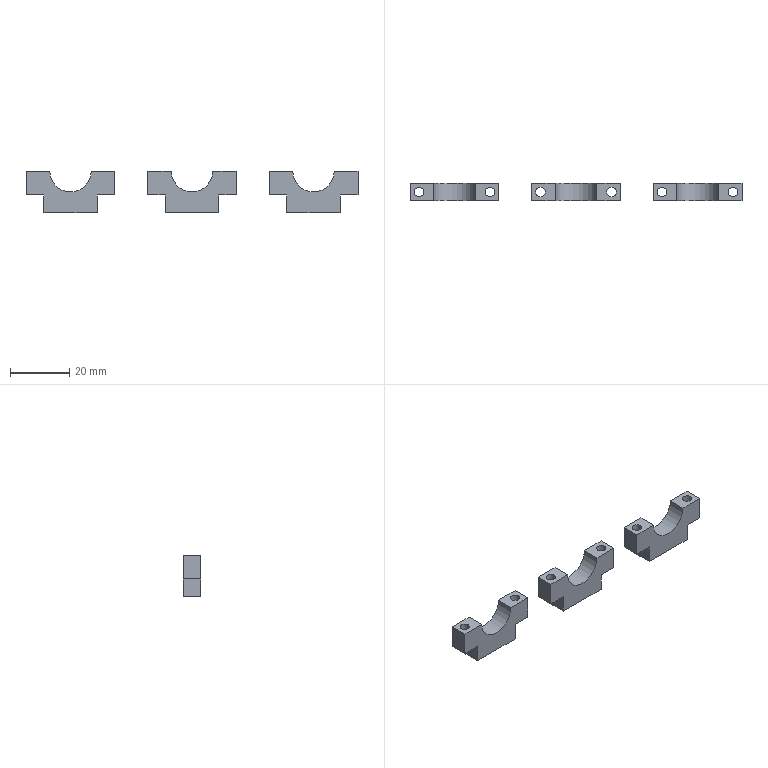Part | 3 solids | 42 faces | box 112 x 6 x 14 mm | volume 4493 mm3 | plane 33 | cylinder 9 | commonest cylinder face diameters 3.2 x6 14 x3
STEP:
#1=CARTESIAN_POINT('',(51.4,0.,-8.));
#2=VERTEX_POINT('',#1);
#3=CARTESIAN_POINT('',(53.,0.,-8.));
#4=DIRECTION('',(0.,0.,1.));
#5=DIRECTION('',(-1.,0.,0.));
#6=AXIS2_PLACEMENT_3D('',#3,#4,#5);
#7=CIRCLE('',#6,1.6);
#8=EDGE_CURVE('',#2,#2,#7,.T.);
#9=ORIENTED_EDGE('',*,*,#8,.F.);
#10=EDGE_LOOP('',(#9));
#11=FACE_BOUND('',#10,.T.);
#12=CARTESIAN_POINT('',(51.4,0.,0.));
#13=VERTEX_POINT('',#12);
#14=CARTESIAN_POINT('',(53.,0.,0.));
#15=DIRECTION('',(0.,0.,1.));
#16=DIRECTION('',(-1.,0.,0.));
#17=AXIS2_PLACEMENT_3D('',#14,#15,#16);
#18=CIRCLE('',#17,1.6);
#19=EDGE_CURVE('',#13,#13,#18,.T.);
#20=ORIENTED_EDGE('',*,*,#19,.T.);
#21=EDGE_LOOP('',(#20));
#22=FACE_BOUND('',#21,.T.);
#23=CARTESIAN_POINT('',(53.,0.,0.));
#24=DIRECTION('',(0.,0.,1.));
#25=DIRECTION('',(1.,0.,0.));
#26=AXIS2_PLACEMENT_3D('',#23,#24,#25);
#27=CYLINDRICAL_SURFACE('',#26,1.6);
#28=ADVANCED_FACE('',(#11,#22),#27,.F.);
#29=CARTESIAN_POINT('',(30.6,0.,-8.));
#30=VERTEX_POINT('',#29);
#31=CARTESIAN_POINT('',(29.,0.,-8.));
#32=DIRECTION('',(0.,0.,1.));
#33=DIRECTION('',(1.,0.,0.));
#34=AXIS2_PLACEMENT_3D('',#31,#32,#33);
#35=CIRCLE('',#34,1.6);
#36=EDGE_CURVE('',#30,#30,#35,.T.);
#37=ORIENTED_EDGE('',*,*,#36,.F.);
#38=EDGE_LOOP('',(#37));
#39=FACE_BOUND('',#38,.T.);
#40=CARTESIAN_POINT('',(30.6,0.,0.));
#41=VERTEX_POINT('',#40);
#42=CARTESIAN_POINT('',(29.,0.,0.));
#43=DIRECTION('',(0.,0.,1.));
#44=DIRECTION('',(1.,0.,0.));
#45=AXIS2_PLACEMENT_3D('',#42,#43,#44);
#46=CIRCLE('',#45,1.6);
#47=EDGE_CURVE('',#41,#41,#46,.T.);
#48=ORIENTED_EDGE('',*,*,#47,.T.);
#49=EDGE_LOOP('',(#48));
#50=FACE_BOUND('',#49,.T.);
#51=CARTESIAN_POINT('',(29.,0.,0.));
#52=DIRECTION('',(0.,0.,1.));
#53=DIRECTION('',(1.,0.,0.));
#54=AXIS2_PLACEMENT_3D('',#51,#52,#53);
#55=CYLINDRICAL_SURFACE('',#54,1.6);
#56=ADVANCED_FACE('',(#39,#50),#55,.F.);
#57=CARTESIAN_POINT('',(26.,3.,-8.));
#58=VERTEX_POINT('',#57);
#59=CARTESIAN_POINT('',(26.,3.,0.));
#60=VERTEX_POINT('',#59);
#61=CARTESIAN_POINT('',(26.,3.,-8.));
#62=DIRECTION('',(0.,0.,1.));
#63=VECTOR('',#62,1000.);
#64=LINE('',#61,#63);
#65=EDGE_CURVE('',#58,#60,#64,.T.);
#66=ORIENTED_EDGE('',*,*,#65,.T.);
#67=CARTESIAN_POINT('',(34.,3.,0.));
#68=VERTEX_POINT('',#67);
#69=CARTESIAN_POINT('',(41.,3.,0.));
#70=DIRECTION('',(1.,0.,0.));
#71=VECTOR('',#70,1000.);
#72=LINE('',#69,#71);
#73=EDGE_CURVE('',#60,#68,#72,.T.);
#74=ORIENTED_EDGE('',*,*,#73,.T.);
#75=CARTESIAN_POINT('',(48.,3.,0.));
#76=VERTEX_POINT('',#75);
#77=CARTESIAN_POINT('',(41.,3.,0.));
#78=DIRECTION('',(0.,-1.,0.));
#79=DIRECTION('',(-1.,0.,0.));
#80=AXIS2_PLACEMENT_3D('',#77,#78,#79);
#81=CIRCLE('',#80,7.);
#82=EDGE_CURVE('',#68,#76,#81,.T.);
#83=ORIENTED_EDGE('',*,*,#82,.T.);
#84=CARTESIAN_POINT('',(56.,3.,0.));
#85=VERTEX_POINT('',#84);
#86=CARTESIAN_POINT('',(48.,3.,0.));
#87=DIRECTION('',(1.,0.,0.));
#88=VECTOR('',#87,1000.);
#89=LINE('',#86,#88);
#90=EDGE_CURVE('',#76,#85,#89,.T.);
#91=ORIENTED_EDGE('',*,*,#90,.T.);
#92=CARTESIAN_POINT('',(56.,3.,-8.));
#93=VERTEX_POINT('',#92);
#94=CARTESIAN_POINT('',(56.,3.,0.));
#95=DIRECTION('',(0.,0.,-1.));
#96=VECTOR('',#95,1000.);
#97=LINE('',#94,#96);
#98=EDGE_CURVE('',#85,#93,#97,.T.);
#99=ORIENTED_EDGE('',*,*,#98,.T.);
#100=CARTESIAN_POINT('',(50.,3.,-8.));
#101=VERTEX_POINT('',#100);
#102=CARTESIAN_POINT('',(56.,3.,-8.));
#103=DIRECTION('',(-1.,0.,0.));
#104=VECTOR('',#103,1000.);
#105=LINE('',#102,#104);
#106=EDGE_CURVE('',#93,#101,#105,.T.);
#107=ORIENTED_EDGE('',*,*,#106,.T.);
#108=CARTESIAN_POINT('',(50.,3.,-14.));
#109=VERTEX_POINT('',#108);
#110=CARTESIAN_POINT('',(50.,3.,-14.));
#111=DIRECTION('',(0.,0.,1.));
#112=VECTOR('',#111,1000.);
#113=LINE('',#110,#112);
#114=EDGE_CURVE('',#109,#101,#113,.T.);
#115=ORIENTED_EDGE('',*,*,#114,.F.);
#116=CARTESIAN_POINT('',(32.,3.,-14.));
#117=VERTEX_POINT('',#116);
#118=CARTESIAN_POINT('',(50.,3.,-14.));
#119=DIRECTION('',(-1.,0.,0.));
#120=VECTOR('',#119,1000.);
#121=LINE('',#118,#120);
#122=EDGE_CURVE('',#109,#117,#121,.T.);
#123=ORIENTED_EDGE('',*,*,#122,.T.);
#124=CARTESIAN_POINT('',(32.,3.,-8.));
#125=VERTEX_POINT('',#124);
#126=CARTESIAN_POINT('',(32.,3.,-8.));
#127=DIRECTION('',(0.,0.,-1.));
#128=VECTOR('',#127,1000.);
#129=LINE('',#126,#128);
#130=EDGE_CURVE('',#125,#117,#129,.T.);
#131=ORIENTED_EDGE('',*,*,#130,.F.);
#132=CARTESIAN_POINT('',(50.,3.,-8.));
#133=DIRECTION('',(1.,0.,0.));
#134=VECTOR('',#133,1000.);
#135=LINE('',#132,#134);
#136=EDGE_CURVE('',#58,#125,#135,.T.);
#137=ORIENTED_EDGE('',*,*,#136,.F.);
#138=EDGE_LOOP('',(#66,#74,#83,#91,#99,#107,#115,#123,#131,#137));
#139=FACE_BOUND('',#138,.T.);
#140=CARTESIAN_POINT('',(41.,3.,0.));
#141=DIRECTION('',(0.,1.,0.));
#142=DIRECTION('',(1.,0.,0.));
#143=AXIS2_PLACEMENT_3D('',#140,#141,#142);
#144=PLANE('',#143);
#145=ADVANCED_FACE('',(#139),#144,.T.);
#146=CARTESIAN_POINT('',(26.,-3.,-8.));
#147=VERTEX_POINT('',#146);
#148=CARTESIAN_POINT('',(26.,-3.,0.));
#149=VERTEX_POINT('',#148);
#150=CARTESIAN_POINT('',(26.,-3.,-8.));
#151=DIRECTION('',(0.,0.,1.));
#152=VECTOR('',#151,1000.);
#153=LINE('',#150,#152);
#154=EDGE_CURVE('',#147,#149,#153,.T.);
#155=ORIENTED_EDGE('',*,*,#154,.T.);
#156=CARTESIAN_POINT('',(26.,-3.,0.));
#157=DIRECTION('',(0.,1.,0.));
#158=VECTOR('',#157,1000.);
#159=LINE('',#156,#158);
#160=EDGE_CURVE('',#149,#60,#159,.T.);
#161=ORIENTED_EDGE('',*,*,#160,.T.);
#162=ORIENTED_EDGE('',*,*,#65,.F.);
#163=CARTESIAN_POINT('',(26.,3.,-8.));
#164=DIRECTION('',(0.,1.,0.));
#165=VECTOR('',#164,1000.);
#166=LINE('',#163,#165);
#167=EDGE_CURVE('',#147,#58,#166,.T.);
#168=ORIENTED_EDGE('',*,*,#167,.F.);
#169=EDGE_LOOP('',(#155,#161,#162,#168));
#170=FACE_BOUND('',#169,.T.);
#171=CARTESIAN_POINT('',(26.,-3.,-14.));
#172=DIRECTION('',(-1.,0.,0.));
#173=DIRECTION('',(0.,0.,1.));
#174=AXIS2_PLACEMENT_3D('',#171,#172,#173);
#175=PLANE('',#174);
#176=ADVANCED_FACE('',(#170),#175,.T.);
#177=ORIENTED_EDGE('',*,*,#47,.F.);
#178=EDGE_LOOP('',(#177));
#179=FACE_BOUND('',#178,.T.);
#180=CARTESIAN_POINT('',(34.,-3.,0.));
#181=VERTEX_POINT('',#180);
#182=CARTESIAN_POINT('',(34.,-3.,0.));
#183=DIRECTION('',(0.,1.,0.));
#184=VECTOR('',#183,1000.);
#185=LINE('',#182,#184);
#186=EDGE_CURVE('',#181,#68,#185,.T.);
#187=ORIENTED_EDGE('',*,*,#186,.T.);
#188=ORIENTED_EDGE('',*,*,#73,.F.);
#189=ORIENTED_EDGE('',*,*,#160,.F.);
#190=CARTESIAN_POINT('',(48.,-3.,0.));
#191=DIRECTION('',(1.,0.,0.));
#192=VECTOR('',#191,1000.);
#193=LINE('',#190,#192);
#194=EDGE_CURVE('',#149,#181,#193,.T.);
#195=ORIENTED_EDGE('',*,*,#194,.T.);
#196=EDGE_LOOP('',(#187,#188,#189,#195));
#197=FACE_BOUND('',#196,.T.);
#198=CARTESIAN_POINT('',(48.,-3.,0.));
#199=DIRECTION('',(0.,0.,1.));
#200=DIRECTION('',(1.,0.,0.));
#201=AXIS2_PLACEMENT_3D('',#198,#199,#200);
#202=PLANE('',#201);
#203=ADVANCED_FACE('',(#179,#197),#202,.T.);
#204=CARTESIAN_POINT('',(48.,-3.,0.));
#205=VERTEX_POINT('',#204);
#206=CARTESIAN_POINT('',(48.,-3.,0.));
#207=DIRECTION('',(0.,1.,0.));
#208=VECTOR('',#207,1000.);
#209=LINE('',#206,#208);
#210=EDGE_CURVE('',#205,#76,#209,.T.);
#211=ORIENTED_EDGE('',*,*,#210,.T.);
#212=ORIENTED_EDGE('',*,*,#82,.F.);
#213=ORIENTED_EDGE('',*,*,#186,.F.);
#214=CARTESIAN_POINT('',(41.,-3.,0.));
#215=DIRECTION('',(0.,-1.,0.));
#216=DIRECTION('',(-1.,0.,0.));
#217=AXIS2_PLACEMENT_3D('',#214,#215,#216);
#218=CIRCLE('',#217,7.);
#219=EDGE_CURVE('',#181,#205,#218,.T.);
#220=ORIENTED_EDGE('',*,*,#219,.T.);
#221=EDGE_LOOP('',(#211,#212,#213,#220));
#222=FACE_BOUND('',#221,.T.);
#223=CARTESIAN_POINT('',(41.,-3.,0.));
#224=DIRECTION('',(0.,1.,0.));
#225=DIRECTION('',(1.,0.,0.));
#226=AXIS2_PLACEMENT_3D('',#223,#224,#225);
#227=CYLINDRICAL_SURFACE('',#226,7.);
#228=ADVANCED_FACE('',(#222),#227,.F.);
#229=ORIENTED_EDGE('',*,*,#19,.F.);
#230=EDGE_LOOP('',(#229));
#231=FACE_BOUND('',#230,.T.);
#232=CARTESIAN_POINT('',(56.,-3.,0.));
#233=VERTEX_POINT('',#232);
#234=CARTESIAN_POINT('',(56.,-3.,0.));
#235=DIRECTION('',(0.,1.,0.));
#236=VECTOR('',#235,1000.);
#237=LINE('',#234,#236);
#238=EDGE_CURVE('',#233,#85,#237,.T.);
#239=ORIENTED_EDGE('',*,*,#238,.T.);
#240=ORIENTED_EDGE('',*,*,#90,.F.);
#241=ORIENTED_EDGE('',*,*,#210,.F.);
#242=CARTESIAN_POINT('',(48.,-3.,0.));
#243=DIRECTION('',(1.,0.,0.));
#244=VECTOR('',#243,1000.);
#245=LINE('',#242,#244);
#246=EDGE_CURVE('',#205,#233,#245,.T.);
#247=ORIENTED_EDGE('',*,*,#246,.T.);
#248=EDGE_LOOP('',(#239,#240,#241,#247));
#249=FACE_BOUND('',#248,.T.);
#250=CARTESIAN_POINT('',(48.,-3.,0.));
#251=DIRECTION('',(0.,0.,1.));
#252=DIRECTION('',(1.,0.,0.));
#253=AXIS2_PLACEMENT_3D('',#250,#251,#252);
#254=PLANE('',#253);
#255=ADVANCED_FACE('',(#231,#249),#254,.T.);
#256=ORIENTED_EDGE('',*,*,#98,.F.);
#257=ORIENTED_EDGE('',*,*,#238,.F.);
#258=CARTESIAN_POINT('',(56.,-3.,-8.));
#259=VERTEX_POINT('',#258);
#260=CARTESIAN_POINT('',(56.,-3.,0.));
#261=DIRECTION('',(0.,0.,-1.));
#262=VECTOR('',#261,1000.);
#263=LINE('',#260,#262);
#264=EDGE_CURVE('',#233,#259,#263,.T.);
#265=ORIENTED_EDGE('',*,*,#264,.T.);
#266=CARTESIAN_POINT('',(56.,-3.,-8.));
#267=DIRECTION('',(0.,1.,0.));
#268=VECTOR('',#267,1000.);
#269=LINE('',#266,#268);
#270=EDGE_CURVE('',#259,#93,#269,.T.);
#271=ORIENTED_EDGE('',*,*,#270,.T.);
#272=EDGE_LOOP('',(#256,#257,#265,#271));
#273=FACE_BOUND('',#272,.T.);
#274=CARTESIAN_POINT('',(56.,-3.,0.));
#275=DIRECTION('',(1.,0.,0.));
#276=DIRECTION('',(0.,0.,-1.));
#277=AXIS2_PLACEMENT_3D('',#274,#275,#276);
#278=PLANE('',#277);
#279=ADVANCED_FACE('',(#273),#278,.T.);
#280=ORIENTED_EDGE('',*,*,#8,.T.);
#281=EDGE_LOOP('',(#280));
#282=FACE_BOUND('',#281,.T.);
#283=CARTESIAN_POINT('',(50.,-3.,-8.));
#284=VERTEX_POINT('',#283);
#285=CARTESIAN_POINT('',(50.,3.,-8.));
#286=DIRECTION('',(0.,-1.,0.));
#287=VECTOR('',#286,1000.);
#288=LINE('',#285,#287);
#289=EDGE_CURVE('',#101,#284,#288,.T.);
#290=ORIENTED_EDGE('',*,*,#289,.F.);
#291=ORIENTED_EDGE('',*,*,#106,.F.);
#292=ORIENTED_EDGE('',*,*,#270,.F.);
#293=CARTESIAN_POINT('',(56.,-3.,-8.));
#294=DIRECTION('',(-1.,0.,0.));
#295=VECTOR('',#294,1000.);
#296=LINE('',#293,#295);
#297=EDGE_CURVE('',#259,#284,#296,.T.);
#298=ORIENTED_EDGE('',*,*,#297,.T.);
#299=EDGE_LOOP('',(#290,#291,#292,#298));
#300=FACE_BOUND('',#299,.T.);
#301=CARTESIAN_POINT('',(50.,3.,-8.));
#302=DIRECTION('',(0.,0.,1.));
#303=DIRECTION('',(1.,0.,0.));
#304=AXIS2_PLACEMENT_3D('',#301,#302,#303);
#305=PLANE('',#304);
#306=ADVANCED_FACE('',(#282,#300),#305,.F.);
#307=CARTESIAN_POINT('',(50.,-3.,-14.));
#308=VERTEX_POINT('',#307);
#309=CARTESIAN_POINT('',(50.,-3.,-14.));
#310=DIRECTION('',(0.,1.,0.));
#311=VECTOR('',#310,1000.);
#312=LINE('',#309,#311);
#313=EDGE_CURVE('',#308,#109,#312,.T.);
#314=ORIENTED_EDGE('',*,*,#313,.T.);
#315=ORIENTED_EDGE('',*,*,#114,.T.);
#316=ORIENTED_EDGE('',*,*,#289,.T.);
#317=CARTESIAN_POINT('',(50.,-3.,-14.));
#318=DIRECTION('',(0.,0.,1.));
#319=VECTOR('',#318,1000.);
#320=LINE('',#317,#319);
#321=EDGE_CURVE('',#308,#284,#320,.T.);
#322=ORIENTED_EDGE('',*,*,#321,.F.);
#323=EDGE_LOOP('',(#314,#315,#316,#322));
#324=FACE_BOUND('',#323,.T.);
#325=CARTESIAN_POINT('',(50.,3.,-14.));
#326=DIRECTION('',(-1.,0.,0.));
#327=DIRECTION('',(0.,0.,1.));
#328=AXIS2_PLACEMENT_3D('',#325,#326,#327);
#329=PLANE('',#328);
#330=ADVANCED_FACE('',(#324),#329,.F.);
#331=ORIENTED_EDGE('',*,*,#122,.F.);
#332=ORIENTED_EDGE('',*,*,#313,.F.);
#333=CARTESIAN_POINT('',(32.,-3.,-14.));
#334=VERTEX_POINT('',#333);
#335=CARTESIAN_POINT('',(50.,-3.,-14.));
#336=DIRECTION('',(-1.,0.,0.));
#337=VECTOR('',#336,1000.);
#338=LINE('',#335,#337);
#339=EDGE_CURVE('',#308,#334,#338,.T.);
#340=ORIENTED_EDGE('',*,*,#339,.T.);
#341=CARTESIAN_POINT('',(32.,-3.,-14.));
#342=DIRECTION('',(0.,1.,0.));
#343=VECTOR('',#342,1000.);
#344=LINE('',#341,#343);
#345=EDGE_CURVE('',#334,#117,#344,.T.);
#346=ORIENTED_EDGE('',*,*,#345,.T.);
#347=EDGE_LOOP('',(#331,#332,#340,#346));
#348=FACE_BOUND('',#347,.T.);
#349=CARTESIAN_POINT('',(56.,-3.,-14.));
#350=DIRECTION('',(0.,0.,-1.));
#351=DIRECTION('',(-1.,0.,0.));
#352=AXIS2_PLACEMENT_3D('',#349,#350,#351);
#353=PLANE('',#352);
#354=ADVANCED_FACE('',(#348),#353,.T.);
#355=CARTESIAN_POINT('',(32.,-3.,-8.));
#356=VERTEX_POINT('',#355);
#357=CARTESIAN_POINT('',(32.,3.,-8.));
#358=DIRECTION('',(0.,-1.,0.));
#359=VECTOR('',#358,1000.);
#360=LINE('',#357,#359);
#361=EDGE_CURVE('',#125,#356,#360,.T.);
#362=ORIENTED_EDGE('',*,*,#361,.F.);
#363=ORIENTED_EDGE('',*,*,#130,.T.);
#364=ORIENTED_EDGE('',*,*,#345,.F.);
#365=CARTESIAN_POINT('',(32.,-3.,-8.));
#366=DIRECTION('',(0.,0.,-1.));
#367=VECTOR('',#366,1000.);
#368=LINE('',#365,#367);
#369=EDGE_CURVE('',#356,#334,#368,.T.);
#370=ORIENTED_EDGE('',*,*,#369,.F.);
#371=EDGE_LOOP('',(#362,#363,#364,#370));
#372=FACE_BOUND('',#371,.T.);
#373=CARTESIAN_POINT('',(32.,3.,-8.));
#374=DIRECTION('',(1.,0.,0.));
#375=DIRECTION('',(0.,0.,-1.));
#376=AXIS2_PLACEMENT_3D('',#373,#374,#375);
#377=PLANE('',#376);
#378=ADVANCED_FACE('',(#372),#377,.F.);
#379=ORIENTED_EDGE('',*,*,#36,.T.);
#380=EDGE_LOOP('',(#379));
#381=FACE_BOUND('',#380,.T.);
#382=ORIENTED_EDGE('',*,*,#167,.T.);
#383=ORIENTED_EDGE('',*,*,#136,.T.);
#384=ORIENTED_EDGE('',*,*,#361,.T.);
#385=CARTESIAN_POINT('',(41.,-3.,-8.));
#386=DIRECTION('',(1.,0.,0.));
#387=VECTOR('',#386,1000.);
#388=LINE('',#385,#387);
#389=EDGE_CURVE('',#147,#356,#388,.T.);
#390=ORIENTED_EDGE('',*,*,#389,.F.);
#391=EDGE_LOOP('',(#382,#383,#384,#390));
#392=FACE_BOUND('',#391,.T.);
#393=CARTESIAN_POINT('',(50.,3.,-8.));
#394=DIRECTION('',(0.,0.,1.));
#395=DIRECTION('',(1.,0.,0.));
#396=AXIS2_PLACEMENT_3D('',#393,#394,#395);
#397=PLANE('',#396);
#398=ADVANCED_FACE('',(#381,#392),#397,.F.);
#399=ORIENTED_EDGE('',*,*,#369,.T.);
#400=ORIENTED_EDGE('',*,*,#339,.F.);
#401=ORIENTED_EDGE('',*,*,#321,.T.);
#402=ORIENTED_EDGE('',*,*,#297,.F.);
#403=ORIENTED_EDGE('',*,*,#264,.F.);
#404=ORIENTED_EDGE('',*,*,#246,.F.);
#405=ORIENTED_EDGE('',*,*,#219,.F.);
#406=ORIENTED_EDGE('',*,*,#194,.F.);
#407=ORIENTED_EDGE('',*,*,#154,.F.);
#408=ORIENTED_EDGE('',*,*,#389,.T.);
#409=EDGE_LOOP('',(#399,#400,#401,#402,#403,#404,#405,#406,#407,#408));
#410=FACE_BOUND('',#409,.T.);
#411=CARTESIAN_POINT('',(41.,-3.,0.));
#412=DIRECTION('',(0.,1.,0.));
#413=DIRECTION('',(1.,0.,0.));
#414=AXIS2_PLACEMENT_3D('',#411,#412,#413);
#415=PLANE('',#414);
#416=ADVANCED_FACE('',(#410),#415,.F.);
#417=CLOSED_SHELL('',(#28,#56,#145,#176,#203,#228,#255,#279,#306,#330,#354,#378,#398,#416));
#418=MANIFOLD_SOLID_BREP('',#417);
#419=CARTESIAN_POINT('',(10.4,0.,-8.));
#420=VERTEX_POINT('',#419);
#421=CARTESIAN_POINT('',(12.,0.,-8.));
#422=DIRECTION('',(0.,0.,1.));
#423=DIRECTION('',(-1.,0.,0.));
#424=AXIS2_PLACEMENT_3D('',#421,#422,#423);
#425=CIRCLE('',#424,1.6);
#426=EDGE_CURVE('',#420,#420,#425,.T.);
#427=ORIENTED_EDGE('',*,*,#426,.F.);
#428=EDGE_LOOP('',(#427));
#429=FACE_BOUND('',#428,.T.);
#430=CARTESIAN_POINT('',(10.4,0.,0.));
#431=VERTEX_POINT('',#430);
#432=CARTESIAN_POINT('',(12.,0.,0.));
#433=DIRECTION('',(0.,0.,1.));
#434=DIRECTION('',(-1.,0.,0.));
#435=AXIS2_PLACEMENT_3D('',#432,#433,#434);
#436=CIRCLE('',#435,1.6);
#437=EDGE_CURVE('',#431,#431,#436,.T.);
#438=ORIENTED_EDGE('',*,*,#437,.T.);
#439=EDGE_LOOP('',(#438));
#440=FACE_BOUND('',#439,.T.);
#441=CARTESIAN_POINT('',(12.,0.,0.));
#442=DIRECTION('',(0.,0.,1.));
#443=DIRECTION('',(1.,0.,0.));
#444=AXIS2_PLACEMENT_3D('',#441,#442,#443);
#445=CYLINDRICAL_SURFACE('',#444,1.6);
#446=ADVANCED_FACE('',(#429,#440),#445,.F.);
#447=CARTESIAN_POINT('',(-10.4,0.,-8.));
#448=VERTEX_POINT('',#447);
#449=CARTESIAN_POINT('',(-12.,0.,-8.));
#450=DIRECTION('',(0.,0.,1.));
#451=DIRECTION('',(1.,0.,0.));
#452=AXIS2_PLACEMENT_3D('',#449,#450,#451);
#453=CIRCLE('',#452,1.6);
#454=EDGE_CURVE('',#448,#448,#453,.T.);
#455=ORIENTED_EDGE('',*,*,#454,.F.);
#456=EDGE_LOOP('',(#455));
#457=FACE_BOUND('',#456,.T.);
#458=CARTESIAN_POINT('',(-10.4,0.,0.));
#459=VERTEX_POINT('',#458);
#460=CARTESIAN_POINT('',(-12.,0.,0.));
#461=DIRECTION('',(0.,0.,1.));
#462=DIRECTION('',(1.,0.,0.));
#463=AXIS2_PLACEMENT_3D('',#460,#461,#462);
#464=CIRCLE('',#463,1.6);
#465=EDGE_CURVE('',#459,#459,#464,.T.);
#466=ORIENTED_EDGE('',*,*,#465,.T.);
#467=EDGE_LOOP('',(#466));
#468=FACE_BOUND('',#467,.T.);
#469=CARTESIAN_POINT('',(-12.,0.,0.));
#470=DIRECTION('',(0.,0.,1.));
#471=DIRECTION('',(1.,0.,0.));
#472=AXIS2_PLACEMENT_3D('',#469,#470,#471);
#473=CYLINDRICAL_SURFACE('',#472,1.6);
#474=ADVANCED_FACE('',(#457,#468),#473,.F.);
#475=CARTESIAN_POINT('',(-15.,3.,-8.));
#476=VERTEX_POINT('',#475);
#477=CARTESIAN_POINT('',(-15.,3.,0.));
#478=VERTEX_POINT('',#477);
#479=CARTESIAN_POINT('',(-15.,3.,-8.));
#480=DIRECTION('',(0.,0.,1.));
#481=VECTOR('',#480,1000.);
#482=LINE('',#479,#481);
#483=EDGE_CURVE('',#476,#478,#482,.T.);
#484=ORIENTED_EDGE('',*,*,#483,.T.);
#485=CARTESIAN_POINT('',(-7.,3.,0.));
#486=VERTEX_POINT('',#485);
#487=CARTESIAN_POINT('',(0.,3.,0.));
#488=DIRECTION('',(1.,0.,0.));
#489=VECTOR('',#488,1000.);
#490=LINE('',#487,#489);
#491=EDGE_CURVE('',#478,#486,#490,.T.);
#492=ORIENTED_EDGE('',*,*,#491,.T.);
#493=CARTESIAN_POINT('',(7.,3.,0.));
#494=VERTEX_POINT('',#493);
#495=CARTESIAN_POINT('',(0.,3.,0.));
#496=DIRECTION('',(0.,-1.,0.));
#497=DIRECTION('',(-1.,0.,0.));
#498=AXIS2_PLACEMENT_3D('',#495,#496,#497);
#499=CIRCLE('',#498,7.);
#500=EDGE_CURVE('',#486,#494,#499,.T.);
#501=ORIENTED_EDGE('',*,*,#500,.T.);
#502=CARTESIAN_POINT('',(15.,3.,0.));
#503=VERTEX_POINT('',#502);
#504=CARTESIAN_POINT('',(7.,3.,0.));
#505=DIRECTION('',(1.,0.,0.));
#506=VECTOR('',#505,1000.);
#507=LINE('',#504,#506);
#508=EDGE_CURVE('',#494,#503,#507,.T.);
#509=ORIENTED_EDGE('',*,*,#508,.T.);
#510=CARTESIAN_POINT('',(15.,3.,-8.));
#511=VERTEX_POINT('',#510);
#512=CARTESIAN_POINT('',(15.,3.,0.));
#513=DIRECTION('',(0.,0.,-1.));
#514=VECTOR('',#513,1000.);
#515=LINE('',#512,#514);
#516=EDGE_CURVE('',#503,#511,#515,.T.);
#517=ORIENTED_EDGE('',*,*,#516,.T.);
#518=CARTESIAN_POINT('',(9.,3.,-8.));
#519=VERTEX_POINT('',#518);
#520=CARTESIAN_POINT('',(15.,3.,-8.));
#521=DIRECTION('',(-1.,0.,0.));
#522=VECTOR('',#521,1000.);
#523=LINE('',#520,#522);
#524=EDGE_CURVE('',#511,#519,#523,.T.);
#525=ORIENTED_EDGE('',*,*,#524,.T.);
#526=CARTESIAN_POINT('',(9.,3.,-14.));
#527=VERTEX_POINT('',#526);
#528=CARTESIAN_POINT('',(9.,3.,-14.));
#529=DIRECTION('',(0.,0.,1.));
#530=VECTOR('',#529,1000.);
#531=LINE('',#528,#530);
#532=EDGE_CURVE('',#527,#519,#531,.T.);
#533=ORIENTED_EDGE('',*,*,#532,.F.);
#534=CARTESIAN_POINT('',(-9.,3.,-14.));
#535=VERTEX_POINT('',#534);
#536=CARTESIAN_POINT('',(9.,3.,-14.));
#537=DIRECTION('',(-1.,0.,0.));
#538=VECTOR('',#537,1000.);
#539=LINE('',#536,#538);
#540=EDGE_CURVE('',#527,#535,#539,.T.);
#541=ORIENTED_EDGE('',*,*,#540,.T.);
#542=CARTESIAN_POINT('',(-9.,3.,-8.));
#543=VERTEX_POINT('',#542);
#544=CARTESIAN_POINT('',(-9.,3.,-8.));
#545=DIRECTION('',(0.,0.,-1.));
#546=VECTOR('',#545,1000.);
#547=LINE('',#544,#546);
#548=EDGE_CURVE('',#543,#535,#547,.T.);
#549=ORIENTED_EDGE('',*,*,#548,.F.);
#550=CARTESIAN_POINT('',(9.,3.,-8.));
#551=DIRECTION('',(1.,0.,0.));
#552=VECTOR('',#551,1000.);
#553=LINE('',#550,#552);
#554=EDGE_CURVE('',#476,#543,#553,.T.);
#555=ORIENTED_EDGE('',*,*,#554,.F.);
#556=EDGE_LOOP('',(#484,#492,#501,#509,#517,#525,#533,#541,#549,#555));
#557=FACE_BOUND('',#556,.T.);
#558=CARTESIAN_POINT('',(0.,3.,0.));
#559=DIRECTION('',(0.,1.,0.));
#560=DIRECTION('',(1.,0.,0.));
#561=AXIS2_PLACEMENT_3D('',#558,#559,#560);
#562=PLANE('',#561);
#563=ADVANCED_FACE('',(#557),#562,.T.);
#564=CARTESIAN_POINT('',(-15.,-3.,-8.));
#565=VERTEX_POINT('',#564);
#566=CARTESIAN_POINT('',(-15.,-3.,0.));
#567=VERTEX_POINT('',#566);
#568=CARTESIAN_POINT('',(-15.,-3.,-8.));
#569=DIRECTION('',(0.,0.,1.));
#570=VECTOR('',#569,1000.);
#571=LINE('',#568,#570);
#572=EDGE_CURVE('',#565,#567,#571,.T.);
#573=ORIENTED_EDGE('',*,*,#572,.T.);
#574=CARTESIAN_POINT('',(-15.,-3.,0.));
#575=DIRECTION('',(0.,1.,0.));
#576=VECTOR('',#575,1000.);
#577=LINE('',#574,#576);
#578=EDGE_CURVE('',#567,#478,#577,.T.);
#579=ORIENTED_EDGE('',*,*,#578,.T.);
#580=ORIENTED_EDGE('',*,*,#483,.F.);
#581=CARTESIAN_POINT('',(-15.,3.,-8.));
#582=DIRECTION('',(0.,1.,0.));
#583=VECTOR('',#582,1000.);
#584=LINE('',#581,#583);
#585=EDGE_CURVE('',#565,#476,#584,.T.);
#586=ORIENTED_EDGE('',*,*,#585,.F.);
#587=EDGE_LOOP('',(#573,#579,#580,#586));
#588=FACE_BOUND('',#587,.T.);
#589=CARTESIAN_POINT('',(-15.,-3.,-14.));
#590=DIRECTION('',(-1.,0.,0.));
#591=DIRECTION('',(0.,0.,1.));
#592=AXIS2_PLACEMENT_3D('',#589,#590,#591);
#593=PLANE('',#592);
#594=ADVANCED_FACE('',(#588),#593,.T.);
#595=ORIENTED_EDGE('',*,*,#465,.F.);
#596=EDGE_LOOP('',(#595));
#597=FACE_BOUND('',#596,.T.);
#598=CARTESIAN_POINT('',(-7.,-3.,0.));
#599=VERTEX_POINT('',#598);
#600=CARTESIAN_POINT('',(-7.,-3.,0.));
#601=DIRECTION('',(0.,1.,0.));
#602=VECTOR('',#601,1000.);
#603=LINE('',#600,#602);
#604=EDGE_CURVE('',#599,#486,#603,.T.);
#605=ORIENTED_EDGE('',*,*,#604,.T.);
#606=ORIENTED_EDGE('',*,*,#491,.F.);
#607=ORIENTED_EDGE('',*,*,#578,.F.);
#608=CARTESIAN_POINT('',(7.,-3.,0.));
#609=DIRECTION('',(1.,0.,0.));
#610=VECTOR('',#609,1000.);
#611=LINE('',#608,#610);
#612=EDGE_CURVE('',#567,#599,#611,.T.);
#613=ORIENTED_EDGE('',*,*,#612,.T.);
#614=EDGE_LOOP('',(#605,#606,#607,#613));
#615=FACE_BOUND('',#614,.T.);
#616=CARTESIAN_POINT('',(7.,-3.,0.));
#617=DIRECTION('',(0.,0.,1.));
#618=DIRECTION('',(1.,0.,0.));
#619=AXIS2_PLACEMENT_3D('',#616,#617,#618);
#620=PLANE('',#619);
#621=ADVANCED_FACE('',(#597,#615),#620,.T.);
#622=CARTESIAN_POINT('',(7.,-3.,0.));
#623=VERTEX_POINT('',#622);
#624=CARTESIAN_POINT('',(7.,-3.,0.));
#625=DIRECTION('',(0.,1.,0.));
#626=VECTOR('',#625,1000.);
#627=LINE('',#624,#626);
#628=EDGE_CURVE('',#623,#494,#627,.T.);
#629=ORIENTED_EDGE('',*,*,#628,.T.);
#630=ORIENTED_EDGE('',*,*,#500,.F.);
#631=ORIENTED_EDGE('',*,*,#604,.F.);
#632=CARTESIAN_POINT('',(0.,-3.,0.));
#633=DIRECTION('',(0.,-1.,0.));
#634=DIRECTION('',(-1.,0.,0.));
#635=AXIS2_PLACEMENT_3D('',#632,#633,#634);
#636=CIRCLE('',#635,7.);
#637=EDGE_CURVE('',#599,#623,#636,.T.);
#638=ORIENTED_EDGE('',*,*,#637,.T.);
#639=EDGE_LOOP('',(#629,#630,#631,#638));
#640=FACE_BOUND('',#639,.T.);
#641=CARTESIAN_POINT('',(0.,-3.,0.));
#642=DIRECTION('',(0.,1.,0.));
#643=DIRECTION('',(1.,0.,0.));
#644=AXIS2_PLACEMENT_3D('',#641,#642,#643);
#645=CYLINDRICAL_SURFACE('',#644,7.);
#646=ADVANCED_FACE('',(#640),#645,.F.);
#647=ORIENTED_EDGE('',*,*,#437,.F.);
#648=EDGE_LOOP('',(#647));
#649=FACE_BOUND('',#648,.T.);
#650=CARTESIAN_POINT('',(15.,-3.,0.));
#651=VERTEX_POINT('',#650);
#652=CARTESIAN_POINT('',(15.,-3.,0.));
#653=DIRECTION('',(0.,1.,0.));
#654=VECTOR('',#653,1000.);
#655=LINE('',#652,#654);
#656=EDGE_CURVE('',#651,#503,#655,.T.);
#657=ORIENTED_EDGE('',*,*,#656,.T.);
#658=ORIENTED_EDGE('',*,*,#508,.F.);
#659=ORIENTED_EDGE('',*,*,#628,.F.);
#660=CARTESIAN_POINT('',(7.,-3.,0.));
#661=DIRECTION('',(1.,0.,0.));
#662=VECTOR('',#661,1000.);
#663=LINE('',#660,#662);
#664=EDGE_CURVE('',#623,#651,#663,.T.);
#665=ORIENTED_EDGE('',*,*,#664,.T.);
#666=EDGE_LOOP('',(#657,#658,#659,#665));
#667=FACE_BOUND('',#666,.T.);
#668=CARTESIAN_POINT('',(7.,-3.,0.));
#669=DIRECTION('',(0.,0.,1.));
#670=DIRECTION('',(1.,0.,0.));
#671=AXIS2_PLACEMENT_3D('',#668,#669,#670);
#672=PLANE('',#671);
#673=ADVANCED_FACE('',(#649,#667),#672,.T.);
#674=ORIENTED_EDGE('',*,*,#516,.F.);
#675=ORIENTED_EDGE('',*,*,#656,.F.);
#676=CARTESIAN_POINT('',(15.,-3.,-8.));
#677=VERTEX_POINT('',#676);
#678=CARTESIAN_POINT('',(15.,-3.,0.));
#679=DIRECTION('',(0.,0.,-1.));
#680=VECTOR('',#679,1000.);
#681=LINE('',#678,#680);
#682=EDGE_CURVE('',#651,#677,#681,.T.);
#683=ORIENTED_EDGE('',*,*,#682,.T.);
#684=CARTESIAN_POINT('',(15.,-3.,-8.));
#685=DIRECTION('',(0.,1.,0.));
#686=VECTOR('',#685,1000.);
#687=LINE('',#684,#686);
#688=EDGE_CURVE('',#677,#511,#687,.T.);
#689=ORIENTED_EDGE('',*,*,#688,.T.);
#690=EDGE_LOOP('',(#674,#675,#683,#689));
#691=FACE_BOUND('',#690,.T.);
#692=CARTESIAN_POINT('',(15.,-3.,0.));
#693=DIRECTION('',(1.,0.,0.));
#694=DIRECTION('',(0.,0.,-1.));
#695=AXIS2_PLACEMENT_3D('',#692,#693,#694);
#696=PLANE('',#695);
#697=ADVANCED_FACE('',(#691),#696,.T.);
#698=ORIENTED_EDGE('',*,*,#426,.T.);
#699=EDGE_LOOP('',(#698));
#700=FACE_BOUND('',#699,.T.);
#701=CARTESIAN_POINT('',(9.,-3.,-8.));
#702=VERTEX_POINT('',#701);
#703=CARTESIAN_POINT('',(9.,3.,-8.));
#704=DIRECTION('',(0.,-1.,0.));
#705=VECTOR('',#704,1000.);
#706=LINE('',#703,#705);
#707=EDGE_CURVE('',#519,#702,#706,.T.);
#708=ORIENTED_EDGE('',*,*,#707,.F.);
#709=ORIENTED_EDGE('',*,*,#524,.F.);
#710=ORIENTED_EDGE('',*,*,#688,.F.);
#711=CARTESIAN_POINT('',(15.,-3.,-8.));
#712=DIRECTION('',(-1.,0.,0.));
#713=VECTOR('',#712,1000.);
#714=LINE('',#711,#713);
#715=EDGE_CURVE('',#677,#702,#714,.T.);
#716=ORIENTED_EDGE('',*,*,#715,.T.);
#717=EDGE_LOOP('',(#708,#709,#710,#716));
#718=FACE_BOUND('',#717,.T.);
#719=CARTESIAN_POINT('',(9.,3.,-8.));
#720=DIRECTION('',(0.,0.,1.));
#721=DIRECTION('',(1.,0.,0.));
#722=AXIS2_PLACEMENT_3D('',#719,#720,#721);
#723=PLANE('',#722);
#724=ADVANCED_FACE('',(#700,#718),#723,.F.);
#725=CARTESIAN_POINT('',(9.,-3.,-14.));
#726=VERTEX_POINT('',#725);
#727=CARTESIAN_POINT('',(9.,-3.,-14.));
#728=DIRECTION('',(0.,1.,0.));
#729=VECTOR('',#728,1000.);
#730=LINE('',#727,#729);
#731=EDGE_CURVE('',#726,#527,#730,.T.);
#732=ORIENTED_EDGE('',*,*,#731,.T.);
#733=ORIENTED_EDGE('',*,*,#532,.T.);
#734=ORIENTED_EDGE('',*,*,#707,.T.);
#735=CARTESIAN_POINT('',(9.,-3.,-14.));
#736=DIRECTION('',(0.,0.,1.));
#737=VECTOR('',#736,1000.);
#738=LINE('',#735,#737);
#739=EDGE_CURVE('',#726,#702,#738,.T.);
#740=ORIENTED_EDGE('',*,*,#739,.F.);
#741=EDGE_LOOP('',(#732,#733,#734,#740));
#742=FACE_BOUND('',#741,.T.);
#743=CARTESIAN_POINT('',(9.,3.,-14.));
#744=DIRECTION('',(-1.,0.,0.));
#745=DIRECTION('',(0.,0.,1.));
#746=AXIS2_PLACEMENT_3D('',#743,#744,#745);
#747=PLANE('',#746);
#748=ADVANCED_FACE('',(#742),#747,.F.);
#749=ORIENTED_EDGE('',*,*,#540,.F.);
#750=ORIENTED_EDGE('',*,*,#731,.F.);
#751=CARTESIAN_POINT('',(-9.,-3.,-14.));
#752=VERTEX_POINT('',#751);
#753=CARTESIAN_POINT('',(9.,-3.,-14.));
#754=DIRECTION('',(-1.,0.,0.));
#755=VECTOR('',#754,1000.);
#756=LINE('',#753,#755);
#757=EDGE_CURVE('',#726,#752,#756,.T.);
#758=ORIENTED_EDGE('',*,*,#757,.T.);
#759=CARTESIAN_POINT('',(-9.,-3.,-14.));
#760=DIRECTION('',(0.,1.,0.));
#761=VECTOR('',#760,1000.);
#762=LINE('',#759,#761);
#763=EDGE_CURVE('',#752,#535,#762,.T.);
#764=ORIENTED_EDGE('',*,*,#763,.T.);
#765=EDGE_LOOP('',(#749,#750,#758,#764));
#766=FACE_BOUND('',#765,.T.);
#767=CARTESIAN_POINT('',(15.,-3.,-14.));
#768=DIRECTION('',(0.,0.,-1.));
#769=DIRECTION('',(-1.,0.,0.));
#770=AXIS2_PLACEMENT_3D('',#767,#768,#769);
#771=PLANE('',#770);
#772=ADVANCED_FACE('',(#766),#771,.T.);
#773=CARTESIAN_POINT('',(-9.,-3.,-8.));
#774=VERTEX_POINT('',#773);
#775=CARTESIAN_POINT('',(-9.,3.,-8.));
#776=DIRECTION('',(0.,-1.,0.));
#777=VECTOR('',#776,1000.);
#778=LINE('',#775,#777);
#779=EDGE_CURVE('',#543,#774,#778,.T.);
#780=ORIENTED_EDGE('',*,*,#779,.F.);
#781=ORIENTED_EDGE('',*,*,#548,.T.);
#782=ORIENTED_EDGE('',*,*,#763,.F.);
#783=CARTESIAN_POINT('',(-9.,-3.,-8.));
#784=DIRECTION('',(0.,0.,-1.));
#785=VECTOR('',#784,1000.);
#786=LINE('',#783,#785);
#787=EDGE_CURVE('',#774,#752,#786,.T.);
#788=ORIENTED_EDGE('',*,*,#787,.F.);
#789=EDGE_LOOP('',(#780,#781,#782,#788));
#790=FACE_BOUND('',#789,.T.);
#791=CARTESIAN_POINT('',(-9.,3.,-8.));
#792=DIRECTION('',(1.,0.,0.));
#793=DIRECTION('',(0.,0.,-1.));
#794=AXIS2_PLACEMENT_3D('',#791,#792,#793);
#795=PLANE('',#794);
#796=ADVANCED_FACE('',(#790),#795,.F.);
#797=ORIENTED_EDGE('',*,*,#454,.T.);
#798=EDGE_LOOP('',(#797));
#799=FACE_BOUND('',#798,.T.);
#800=ORIENTED_EDGE('',*,*,#585,.T.);
#801=ORIENTED_EDGE('',*,*,#554,.T.);
#802=ORIENTED_EDGE('',*,*,#779,.T.);
#803=CARTESIAN_POINT('',(0.,-3.,-8.));
#804=DIRECTION('',(1.,0.,0.));
#805=VECTOR('',#804,1000.);
#806=LINE('',#803,#805);
#807=EDGE_CURVE('',#565,#774,#806,.T.);
#808=ORIENTED_EDGE('',*,*,#807,.F.);
#809=EDGE_LOOP('',(#800,#801,#802,#808));
#810=FACE_BOUND('',#809,.T.);
#811=CARTESIAN_POINT('',(9.,3.,-8.));
#812=DIRECTION('',(0.,0.,1.));
#813=DIRECTION('',(1.,0.,0.));
#814=AXIS2_PLACEMENT_3D('',#811,#812,#813);
#815=PLANE('',#814);
#816=ADVANCED_FACE('',(#799,#810),#815,.F.);
#817=ORIENTED_EDGE('',*,*,#787,.T.);
#818=ORIENTED_EDGE('',*,*,#757,.F.);
#819=ORIENTED_EDGE('',*,*,#739,.T.);
#820=ORIENTED_EDGE('',*,*,#715,.F.);
#821=ORIENTED_EDGE('',*,*,#682,.F.);
#822=ORIENTED_EDGE('',*,*,#664,.F.);
#823=ORIENTED_EDGE('',*,*,#637,.F.);
#824=ORIENTED_EDGE('',*,*,#612,.F.);
#825=ORIENTED_EDGE('',*,*,#572,.F.);
#826=ORIENTED_EDGE('',*,*,#807,.T.);
#827=EDGE_LOOP('',(#817,#818,#819,#820,#821,#822,#823,#824,#825,#826));
#828=FACE_BOUND('',#827,.T.);
#829=CARTESIAN_POINT('',(0.,-3.,0.));
#830=DIRECTION('',(0.,1.,0.));
#831=DIRECTION('',(1.,0.,0.));
#832=AXIS2_PLACEMENT_3D('',#829,#830,#831);
#833=PLANE('',#832);
#834=ADVANCED_FACE('',(#828),#833,.F.);
#835=CLOSED_SHELL('',(#446,#474,#563,#594,#621,#646,#673,#697,#724,#748,#772,#796,#816,#834));
#836=MANIFOLD_SOLID_BREP('',#835);
#837=CARTESIAN_POINT('',(92.4,0.,-8.));
#838=VERTEX_POINT('',#837);
#839=CARTESIAN_POINT('',(94.,0.,-8.));
#840=DIRECTION('',(0.,0.,1.));
#841=DIRECTION('',(-1.,0.,0.));
#842=AXIS2_PLACEMENT_3D('',#839,#840,#841);
#843=CIRCLE('',#842,1.6);
#844=EDGE_CURVE('',#838,#838,#843,.T.);
#845=ORIENTED_EDGE('',*,*,#844,.F.);
#846=EDGE_LOOP('',(#845));
#847=FACE_BOUND('',#846,.T.);
#848=CARTESIAN_POINT('',(92.4,0.,0.));
#849=VERTEX_POINT('',#848);
#850=CARTESIAN_POINT('',(94.,0.,0.));
#851=DIRECTION('',(0.,0.,1.));
#852=DIRECTION('',(-1.,0.,0.));
#853=AXIS2_PLACEMENT_3D('',#850,#851,#852);
#854=CIRCLE('',#853,1.6);
#855=EDGE_CURVE('',#849,#849,#854,.T.);
#856=ORIENTED_EDGE('',*,*,#855,.T.);
#857=EDGE_LOOP('',(#856));
#858=FACE_BOUND('',#857,.T.);
#859=CARTESIAN_POINT('',(94.,0.,0.));
#860=DIRECTION('',(0.,0.,1.));
#861=DIRECTION('',(1.,0.,0.));
#862=AXIS2_PLACEMENT_3D('',#859,#860,#861);
#863=CYLINDRICAL_SURFACE('',#862,1.6);
#864=ADVANCED_FACE('',(#847,#858),#863,.F.);
#865=CARTESIAN_POINT('',(71.6,0.,-8.));
#866=VERTEX_POINT('',#865);
#867=CARTESIAN_POINT('',(70.,0.,-8.));
#868=DIRECTION('',(0.,0.,1.));
#869=DIRECTION('',(1.,0.,0.));
#870=AXIS2_PLACEMENT_3D('',#867,#868,#869);
#871=CIRCLE('',#870,1.6);
#872=EDGE_CURVE('',#866,#866,#871,.T.);
#873=ORIENTED_EDGE('',*,*,#872,.F.);
#874=EDGE_LOOP('',(#873));
#875=FACE_BOUND('',#874,.T.);
#876=CARTESIAN_POINT('',(71.6,0.,0.));
#877=VERTEX_POINT('',#876);
#878=CARTESIAN_POINT('',(70.,0.,0.));
#879=DIRECTION('',(0.,0.,1.));
#880=DIRECTION('',(1.,0.,0.));
#881=AXIS2_PLACEMENT_3D('',#878,#879,#880);
#882=CIRCLE('',#881,1.6);
#883=EDGE_CURVE('',#877,#877,#882,.T.);
#884=ORIENTED_EDGE('',*,*,#883,.T.);
#885=EDGE_LOOP('',(#884));
#886=FACE_BOUND('',#885,.T.);
#887=CARTESIAN_POINT('',(70.,0.,0.));
#888=DIRECTION('',(0.,0.,1.));
#889=DIRECTION('',(1.,0.,0.));
#890=AXIS2_PLACEMENT_3D('',#887,#888,#889);
#891=CYLINDRICAL_SURFACE('',#890,1.6);
#892=ADVANCED_FACE('',(#875,#886),#891,.F.);
#893=CARTESIAN_POINT('',(67.,3.,-8.));
#894=VERTEX_POINT('',#893);
#895=CARTESIAN_POINT('',(67.,3.,0.));
#896=VERTEX_POINT('',#895);
#897=CARTESIAN_POINT('',(67.,3.,-8.));
#898=DIRECTION('',(0.,0.,1.));
#899=VECTOR('',#898,1000.);
#900=LINE('',#897,#899);
#901=EDGE_CURVE('',#894,#896,#900,.T.);
#902=ORIENTED_EDGE('',*,*,#901,.T.);
#903=CARTESIAN_POINT('',(75.,3.,0.));
#904=VERTEX_POINT('',#903);
#905=CARTESIAN_POINT('',(82.,3.,0.));
#906=DIRECTION('',(1.,0.,0.));
#907=VECTOR('',#906,1000.);
#908=LINE('',#905,#907);
#909=EDGE_CURVE('',#896,#904,#908,.T.);
#910=ORIENTED_EDGE('',*,*,#909,.T.);
#911=CARTESIAN_POINT('',(89.,3.,0.));
#912=VERTEX_POINT('',#911);
#913=CARTESIAN_POINT('',(82.,3.,0.));
#914=DIRECTION('',(0.,-1.,0.));
#915=DIRECTION('',(-1.,0.,0.));
#916=AXIS2_PLACEMENT_3D('',#913,#914,#915);
#917=CIRCLE('',#916,7.);
#918=EDGE_CURVE('',#904,#912,#917,.T.);
#919=ORIENTED_EDGE('',*,*,#918,.T.);
#920=CARTESIAN_POINT('',(97.,3.,0.));
#921=VERTEX_POINT('',#920);
#922=CARTESIAN_POINT('',(89.,3.,0.));
#923=DIRECTION('',(1.,0.,0.));
#924=VECTOR('',#923,1000.);
#925=LINE('',#922,#924);
#926=EDGE_CURVE('',#912,#921,#925,.T.);
#927=ORIENTED_EDGE('',*,*,#926,.T.);
#928=CARTESIAN_POINT('',(97.,3.,-8.));
#929=VERTEX_POINT('',#928);
#930=CARTESIAN_POINT('',(97.,3.,0.));
#931=DIRECTION('',(0.,0.,-1.));
#932=VECTOR('',#931,1000.);
#933=LINE('',#930,#932);
#934=EDGE_CURVE('',#921,#929,#933,.T.);
#935=ORIENTED_EDGE('',*,*,#934,.T.);
#936=CARTESIAN_POINT('',(91.,3.,-8.));
#937=VERTEX_POINT('',#936);
#938=CARTESIAN_POINT('',(97.,3.,-8.));
#939=DIRECTION('',(-1.,0.,0.));
#940=VECTOR('',#939,1000.);
#941=LINE('',#938,#940);
#942=EDGE_CURVE('',#929,#937,#941,.T.);
#943=ORIENTED_EDGE('',*,*,#942,.T.);
#944=CARTESIAN_POINT('',(91.,3.,-14.));
#945=VERTEX_POINT('',#944);
#946=CARTESIAN_POINT('',(91.,3.,-14.));
#947=DIRECTION('',(0.,0.,1.));
#948=VECTOR('',#947,1000.);
#949=LINE('',#946,#948);
#950=EDGE_CURVE('',#945,#937,#949,.T.);
#951=ORIENTED_EDGE('',*,*,#950,.F.);
#952=CARTESIAN_POINT('',(73.,3.,-14.));
#953=VERTEX_POINT('',#952);
#954=CARTESIAN_POINT('',(91.,3.,-14.));
#955=DIRECTION('',(-1.,0.,0.));
#956=VECTOR('',#955,1000.);
#957=LINE('',#954,#956);
#958=EDGE_CURVE('',#945,#953,#957,.T.);
#959=ORIENTED_EDGE('',*,*,#958,.T.);
#960=CARTESIAN_POINT('',(73.,3.,-8.));
#961=VERTEX_POINT('',#960);
#962=CARTESIAN_POINT('',(73.,3.,-8.));
#963=DIRECTION('',(0.,0.,-1.));
#964=VECTOR('',#963,1000.);
#965=LINE('',#962,#964);
#966=EDGE_CURVE('',#961,#953,#965,.T.);
#967=ORIENTED_EDGE('',*,*,#966,.F.);
#968=CARTESIAN_POINT('',(91.,3.,-8.));
#969=DIRECTION('',(1.,0.,0.));
#970=VECTOR('',#969,1000.);
#971=LINE('',#968,#970);
#972=EDGE_CURVE('',#894,#961,#971,.T.);
#973=ORIENTED_EDGE('',*,*,#972,.F.);
#974=EDGE_LOOP('',(#902,#910,#919,#927,#935,#943,#951,#959,#967,#973));
#975=FACE_BOUND('',#974,.T.);
#976=CARTESIAN_POINT('',(82.,3.,0.));
#977=DIRECTION('',(0.,1.,0.));
#978=DIRECTION('',(1.,0.,0.));
#979=AXIS2_PLACEMENT_3D('',#976,#977,#978);
#980=PLANE('',#979);
#981=ADVANCED_FACE('',(#975),#980,.T.);
#982=CARTESIAN_POINT('',(67.,-3.,-8.));
#983=VERTEX_POINT('',#982);
#984=CARTESIAN_POINT('',(67.,-3.,0.));
#985=VERTEX_POINT('',#984);
#986=CARTESIAN_POINT('',(67.,-3.,-8.));
#987=DIRECTION('',(0.,0.,1.));
#988=VECTOR('',#987,1000.);
#989=LINE('',#986,#988);
#990=EDGE_CURVE('',#983,#985,#989,.T.);
#991=ORIENTED_EDGE('',*,*,#990,.T.);
#992=CARTESIAN_POINT('',(67.,-3.,0.));
#993=DIRECTION('',(0.,1.,0.));
#994=VECTOR('',#993,1000.);
#995=LINE('',#992,#994);
#996=EDGE_CURVE('',#985,#896,#995,.T.);
#997=ORIENTED_EDGE('',*,*,#996,.T.);
#998=ORIENTED_EDGE('',*,*,#901,.F.);
#999=CARTESIAN_POINT('',(67.,3.,-8.));
#1000=DIRECTION('',(0.,1.,0.));
#1001=VECTOR('',#1000,1000.);
#1002=LINE('',#999,#1001);
#1003=EDGE_CURVE('',#983,#894,#1002,.T.);
#1004=ORIENTED_EDGE('',*,*,#1003,.F.);
#1005=EDGE_LOOP('',(#991,#997,#998,#1004));
#1006=FACE_BOUND('',#1005,.T.);
#1007=CARTESIAN_POINT('',(67.,-3.,-14.));
#1008=DIRECTION('',(-1.,0.,0.));
#1009=DIRECTION('',(0.,0.,1.));
#1010=AXIS2_PLACEMENT_3D('',#1007,#1008,#1009);
#1011=PLANE('',#1010);
#1012=ADVANCED_FACE('',(#1006),#1011,.T.);
#1013=ORIENTED_EDGE('',*,*,#883,.F.);
#1014=EDGE_LOOP('',(#1013));
#1015=FACE_BOUND('',#1014,.T.);
#1016=CARTESIAN_POINT('',(75.,-3.,0.));
#1017=VERTEX_POINT('',#1016);
#1018=CARTESIAN_POINT('',(75.,-3.,0.));
#1019=DIRECTION('',(0.,1.,0.));
#1020=VECTOR('',#1019,1000.);
#1021=LINE('',#1018,#1020);
#1022=EDGE_CURVE('',#1017,#904,#1021,.T.);
#1023=ORIENTED_EDGE('',*,*,#1022,.T.);
#1024=ORIENTED_EDGE('',*,*,#909,.F.);
#1025=ORIENTED_EDGE('',*,*,#996,.F.);
#1026=CARTESIAN_POINT('',(89.,-3.,0.));
#1027=DIRECTION('',(1.,0.,0.));
#1028=VECTOR('',#1027,1000.);
#1029=LINE('',#1026,#1028);
#1030=EDGE_CURVE('',#985,#1017,#1029,.T.);
#1031=ORIENTED_EDGE('',*,*,#1030,.T.);
#1032=EDGE_LOOP('',(#1023,#1024,#1025,#1031));
#1033=FACE_BOUND('',#1032,.T.);
#1034=CARTESIAN_POINT('',(89.,-3.,0.));
#1035=DIRECTION('',(0.,0.,1.));
#1036=DIRECTION('',(1.,0.,0.));
#1037=AXIS2_PLACEMENT_3D('',#1034,#1035,#1036);
#1038=PLANE('',#1037);
#1039=ADVANCED_FACE('',(#1015,#1033),#1038,.T.);
#1040=CARTESIAN_POINT('',(89.,-3.,0.));
#1041=VERTEX_POINT('',#1040);
#1042=CARTESIAN_POINT('',(89.,-3.,0.));
#1043=DIRECTION('',(0.,1.,0.));
#1044=VECTOR('',#1043,1000.);
#1045=LINE('',#1042,#1044);
#1046=EDGE_CURVE('',#1041,#912,#1045,.T.);
#1047=ORIENTED_EDGE('',*,*,#1046,.T.);
#1048=ORIENTED_EDGE('',*,*,#918,.F.);
#1049=ORIENTED_EDGE('',*,*,#1022,.F.);
#1050=CARTESIAN_POINT('',(82.,-3.,0.));
#1051=DIRECTION('',(0.,-1.,0.));
#1052=DIRECTION('',(-1.,0.,0.));
#1053=AXIS2_PLACEMENT_3D('',#1050,#1051,#1052);
#1054=CIRCLE('',#1053,7.);
#1055=EDGE_CURVE('',#1017,#1041,#1054,.T.);
#1056=ORIENTED_EDGE('',*,*,#1055,.T.);
#1057=EDGE_LOOP('',(#1047,#1048,#1049,#1056));
#1058=FACE_BOUND('',#1057,.T.);
#1059=CARTESIAN_POINT('',(82.,-3.,0.));
#1060=DIRECTION('',(0.,1.,0.));
#1061=DIRECTION('',(1.,0.,0.));
#1062=AXIS2_PLACEMENT_3D('',#1059,#1060,#1061);
#1063=CYLINDRICAL_SURFACE('',#1062,7.);
#1064=ADVANCED_FACE('',(#1058),#1063,.F.);
#1065=ORIENTED_EDGE('',*,*,#855,.F.);
#1066=EDGE_LOOP('',(#1065));
#1067=FACE_BOUND('',#1066,.T.);
#1068=CARTESIAN_POINT('',(97.,-3.,0.));
#1069=VERTEX_POINT('',#1068);
#1070=CARTESIAN_POINT('',(97.,-3.,0.));
#1071=DIRECTION('',(0.,1.,0.));
#1072=VECTOR('',#1071,1000.);
#1073=LINE('',#1070,#1072);
#1074=EDGE_CURVE('',#1069,#921,#1073,.T.);
#1075=ORIENTED_EDGE('',*,*,#1074,.T.);
#1076=ORIENTED_EDGE('',*,*,#926,.F.);
#1077=ORIENTED_EDGE('',*,*,#1046,.F.);
#1078=CARTESIAN_POINT('',(89.,-3.,0.));
#1079=DIRECTION('',(1.,0.,0.));
#1080=VECTOR('',#1079,1000.);
#1081=LINE('',#1078,#1080);
#1082=EDGE_CURVE('',#1041,#1069,#1081,.T.);
#1083=ORIENTED_EDGE('',*,*,#1082,.T.);
#1084=EDGE_LOOP('',(#1075,#1076,#1077,#1083));
#1085=FACE_BOUND('',#1084,.T.);
#1086=CARTESIAN_POINT('',(89.,-3.,0.));
#1087=DIRECTION('',(0.,0.,1.));
#1088=DIRECTION('',(1.,0.,0.));
#1089=AXIS2_PLACEMENT_3D('',#1086,#1087,#1088);
#1090=PLANE('',#1089);
#1091=ADVANCED_FACE('',(#1067,#1085),#1090,.T.);
#1092=ORIENTED_EDGE('',*,*,#934,.F.);
#1093=ORIENTED_EDGE('',*,*,#1074,.F.);
#1094=CARTESIAN_POINT('',(97.,-3.,-8.));
#1095=VERTEX_POINT('',#1094);
#1096=CARTESIAN_POINT('',(97.,-3.,0.));
#1097=DIRECTION('',(0.,0.,-1.));
#1098=VECTOR('',#1097,1000.);
#1099=LINE('',#1096,#1098);
#1100=EDGE_CURVE('',#1069,#1095,#1099,.T.);
#1101=ORIENTED_EDGE('',*,*,#1100,.T.);
#1102=CARTESIAN_POINT('',(97.,-3.,-8.));
#1103=DIRECTION('',(0.,1.,0.));
#1104=VECTOR('',#1103,1000.);
#1105=LINE('',#1102,#1104);
#1106=EDGE_CURVE('',#1095,#929,#1105,.T.);
#1107=ORIENTED_EDGE('',*,*,#1106,.T.);
#1108=EDGE_LOOP('',(#1092,#1093,#1101,#1107));
#1109=FACE_BOUND('',#1108,.T.);
#1110=CARTESIAN_POINT('',(97.,-3.,0.));
#1111=DIRECTION('',(1.,0.,0.));
#1112=DIRECTION('',(0.,0.,-1.));
#1113=AXIS2_PLACEMENT_3D('',#1110,#1111,#1112);
#1114=PLANE('',#1113);
#1115=ADVANCED_FACE('',(#1109),#1114,.T.);
#1116=ORIENTED_EDGE('',*,*,#844,.T.);
#1117=EDGE_LOOP('',(#1116));
#1118=FACE_BOUND('',#1117,.T.);
#1119=CARTESIAN_POINT('',(91.,-3.,-8.));
#1120=VERTEX_POINT('',#1119);
#1121=CARTESIAN_POINT('',(91.,3.,-8.));
#1122=DIRECTION('',(0.,-1.,0.));
#1123=VECTOR('',#1122,1000.);
#1124=LINE('',#1121,#1123);
#1125=EDGE_CURVE('',#937,#1120,#1124,.T.);
#1126=ORIENTED_EDGE('',*,*,#1125,.F.);
#1127=ORIENTED_EDGE('',*,*,#942,.F.);
#1128=ORIENTED_EDGE('',*,*,#1106,.F.);
#1129=CARTESIAN_POINT('',(97.,-3.,-8.));
#1130=DIRECTION('',(-1.,0.,0.));
#1131=VECTOR('',#1130,1000.);
#1132=LINE('',#1129,#1131);
#1133=EDGE_CURVE('',#1095,#1120,#1132,.T.);
#1134=ORIENTED_EDGE('',*,*,#1133,.T.);
#1135=EDGE_LOOP('',(#1126,#1127,#1128,#1134));
#1136=FACE_BOUND('',#1135,.T.);
#1137=CARTESIAN_POINT('',(91.,3.,-8.));
#1138=DIRECTION('',(0.,0.,1.));
#1139=DIRECTION('',(1.,0.,0.));
#1140=AXIS2_PLACEMENT_3D('',#1137,#1138,#1139);
#1141=PLANE('',#1140);
#1142=ADVANCED_FACE('',(#1118,#1136),#1141,.F.);
#1143=CARTESIAN_POINT('',(91.,-3.,-14.));
#1144=VERTEX_POINT('',#1143);
#1145=CARTESIAN_POINT('',(91.,-3.,-14.));
#1146=DIRECTION('',(0.,1.,0.));
#1147=VECTOR('',#1146,1000.);
#1148=LINE('',#1145,#1147);
#1149=EDGE_CURVE('',#1144,#945,#1148,.T.);
#1150=ORIENTED_EDGE('',*,*,#1149,.T.);
#1151=ORIENTED_EDGE('',*,*,#950,.T.);
#1152=ORIENTED_EDGE('',*,*,#1125,.T.);
#1153=CARTESIAN_POINT('',(91.,-3.,-14.));
#1154=DIRECTION('',(0.,0.,1.));
#1155=VECTOR('',#1154,1000.);
#1156=LINE('',#1153,#1155);
#1157=EDGE_CURVE('',#1144,#1120,#1156,.T.);
#1158=ORIENTED_EDGE('',*,*,#1157,.F.);
#1159=EDGE_LOOP('',(#1150,#1151,#1152,#1158));
#1160=FACE_BOUND('',#1159,.T.);
#1161=CARTESIAN_POINT('',(91.,3.,-14.));
#1162=DIRECTION('',(-1.,0.,0.));
#1163=DIRECTION('',(0.,0.,1.));
#1164=AXIS2_PLACEMENT_3D('',#1161,#1162,#1163);
#1165=PLANE('',#1164);
#1166=ADVANCED_FACE('',(#1160),#1165,.F.);
#1167=ORIENTED_EDGE('',*,*,#958,.F.);
#1168=ORIENTED_EDGE('',*,*,#1149,.F.);
#1169=CARTESIAN_POINT('',(73.,-3.,-14.));
#1170=VERTEX_POINT('',#1169);
#1171=CARTESIAN_POINT('',(91.,-3.,-14.));
#1172=DIRECTION('',(-1.,0.,0.));
#1173=VECTOR('',#1172,1000.);
#1174=LINE('',#1171,#1173);
#1175=EDGE_CURVE('',#1144,#1170,#1174,.T.);
#1176=ORIENTED_EDGE('',*,*,#1175,.T.);
#1177=CARTESIAN_POINT('',(73.,-3.,-14.));
#1178=DIRECTION('',(0.,1.,0.));
#1179=VECTOR('',#1178,1000.);
#1180=LINE('',#1177,#1179);
#1181=EDGE_CURVE('',#1170,#953,#1180,.T.);
#1182=ORIENTED_EDGE('',*,*,#1181,.T.);
#1183=EDGE_LOOP('',(#1167,#1168,#1176,#1182));
#1184=FACE_BOUND('',#1183,.T.);
#1185=CARTESIAN_POINT('',(97.,-3.,-14.));
#1186=DIRECTION('',(0.,0.,-1.));
#1187=DIRECTION('',(-1.,0.,0.));
#1188=AXIS2_PLACEMENT_3D('',#1185,#1186,#1187);
#1189=PLANE('',#1188);
#1190=ADVANCED_FACE('',(#1184),#1189,.T.);
#1191=CARTESIAN_POINT('',(73.,-3.,-8.));
#1192=VERTEX_POINT('',#1191);
#1193=CARTESIAN_POINT('',(73.,3.,-8.));
#1194=DIRECTION('',(0.,-1.,0.));
#1195=VECTOR('',#1194,1000.);
#1196=LINE('',#1193,#1195);
#1197=EDGE_CURVE('',#961,#1192,#1196,.T.);
#1198=ORIENTED_EDGE('',*,*,#1197,.F.);
#1199=ORIENTED_EDGE('',*,*,#966,.T.);
#1200=ORIENTED_EDGE('',*,*,#1181,.F.);
#1201=CARTESIAN_POINT('',(73.,-3.,-8.));
#1202=DIRECTION('',(0.,0.,-1.));
#1203=VECTOR('',#1202,1000.);
#1204=LINE('',#1201,#1203);
#1205=EDGE_CURVE('',#1192,#1170,#1204,.T.);
#1206=ORIENTED_EDGE('',*,*,#1205,.F.);
#1207=EDGE_LOOP('',(#1198,#1199,#1200,#1206));
#1208=FACE_BOUND('',#1207,.T.);
#1209=CARTESIAN_POINT('',(73.,3.,-8.));
#1210=DIRECTION('',(1.,0.,0.));
#1211=DIRECTION('',(0.,0.,-1.));
#1212=AXIS2_PLACEMENT_3D('',#1209,#1210,#1211);
#1213=PLANE('',#1212);
#1214=ADVANCED_FACE('',(#1208),#1213,.F.);
#1215=ORIENTED_EDGE('',*,*,#872,.T.);
#1216=EDGE_LOOP('',(#1215));
#1217=FACE_BOUND('',#1216,.T.);
#1218=ORIENTED_EDGE('',*,*,#1003,.T.);
#1219=ORIENTED_EDGE('',*,*,#972,.T.);
#1220=ORIENTED_EDGE('',*,*,#1197,.T.);
#1221=CARTESIAN_POINT('',(82.,-3.,-8.));
#1222=DIRECTION('',(1.,0.,0.));
#1223=VECTOR('',#1222,1000.);
#1224=LINE('',#1221,#1223);
#1225=EDGE_CURVE('',#983,#1192,#1224,.T.);
#1226=ORIENTED_EDGE('',*,*,#1225,.F.);
#1227=EDGE_LOOP('',(#1218,#1219,#1220,#1226));
#1228=FACE_BOUND('',#1227,.T.);
#1229=CARTESIAN_POINT('',(91.,3.,-8.));
#1230=DIRECTION('',(0.,0.,1.));
#1231=DIRECTION('',(1.,0.,0.));
#1232=AXIS2_PLACEMENT_3D('',#1229,#1230,#1231);
#1233=PLANE('',#1232);
#1234=ADVANCED_FACE('',(#1217,#1228),#1233,.F.);
#1235=ORIENTED_EDGE('',*,*,#1205,.T.);
#1236=ORIENTED_EDGE('',*,*,#1175,.F.);
#1237=ORIENTED_EDGE('',*,*,#1157,.T.);
#1238=ORIENTED_EDGE('',*,*,#1133,.F.);
#1239=ORIENTED_EDGE('',*,*,#1100,.F.);
#1240=ORIENTED_EDGE('',*,*,#1082,.F.);
#1241=ORIENTED_EDGE('',*,*,#1055,.F.);
#1242=ORIENTED_EDGE('',*,*,#1030,.F.);
#1243=ORIENTED_EDGE('',*,*,#990,.F.);
#1244=ORIENTED_EDGE('',*,*,#1225,.T.);
#1245=EDGE_LOOP('',(#1235,#1236,#1237,#1238,#1239,#1240,#1241,#1242,#1243,#1244));
#1246=FACE_BOUND('',#1245,.T.);
#1247=CARTESIAN_POINT('',(82.,-3.,0.));
#1248=DIRECTION('',(0.,1.,0.));
#1249=DIRECTION('',(1.,0.,0.));
#1250=AXIS2_PLACEMENT_3D('',#1247,#1248,#1249);
#1251=PLANE('',#1250);
#1252=ADVANCED_FACE('',(#1246),#1251,.F.);
#1253=CLOSED_SHELL('',(#864,#892,#981,#1012,#1039,#1064,#1091,#1115,#1142,#1166,#1190,#1214,#1234,#1252));
#1254=MANIFOLD_SOLID_BREP('',#1253);
#1255=(LENGTH_UNIT()NAMED_UNIT(*)SI_UNIT(.MILLI.,.METRE.));
#1256=UNCERTAINTY_MEASURE_WITH_UNIT(LENGTH_MEASURE(0.00001),#1255,'','');
#1257=(NAMED_UNIT(*)PLANE_ANGLE_UNIT()SI_UNIT($,.RADIAN.));
#1258=(NAMED_UNIT(*)SI_UNIT($,.STERADIAN.)SOLID_ANGLE_UNIT());
#1259=(GEOMETRIC_REPRESENTATION_CONTEXT(3)GLOBAL_UNCERTAINTY_ASSIGNED_CONTEXT((#1256))GLOBAL_UNIT_ASSIGNED_CONTEXT((#1255,#1257,#1258))REPRESENTATION_CONTEXT('',''));
#1260=ADVANCED_BREP_SHAPE_REPRESENTATION('',(#418,#836,#1254),#1259);